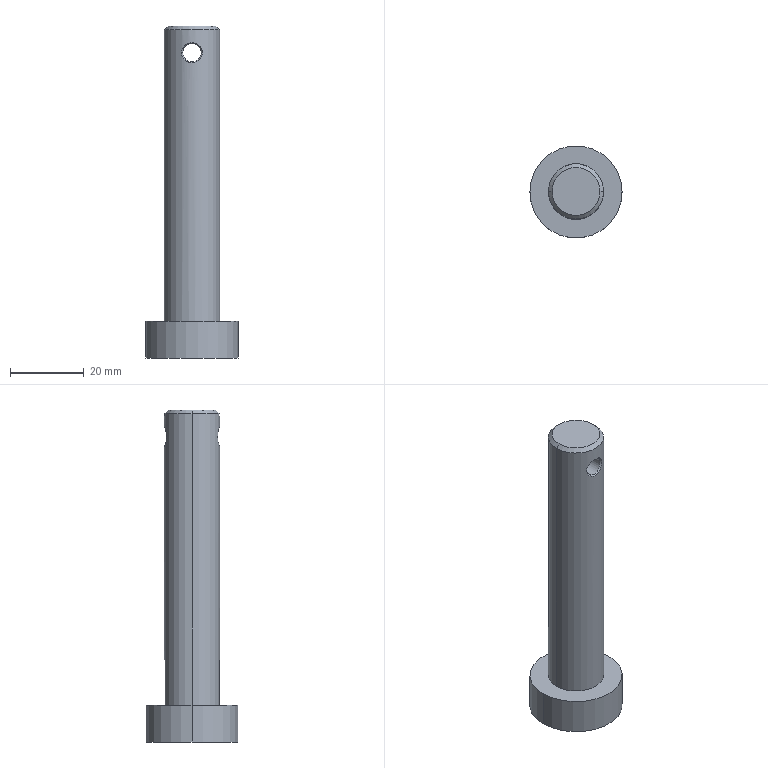Part | SolidWorks | features ICE 4, Chamfer 3, Extrusion 1 | 1 solid | 15 faces | box 25 x 25 x 90 mm | volume 18731 mm3 | cylinder 6 | spline 4 | plane 3 | cone 2 | commonest cylinder face diameters 5 x2 15 x2 25 x2